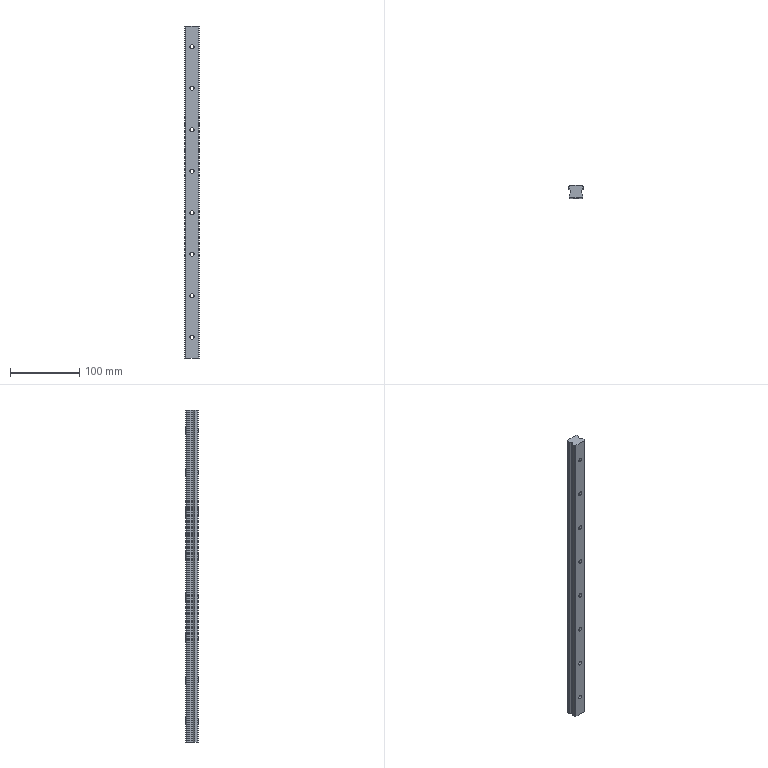Part | SolidWorks | features Chamfer 1, Extrusion 1, HoleWzd 1, LPattern 1 | 1 solid | 68 faces | box 20.703 x 18 x 480 mm | volume 151850 mm3 | cylinder 42 | plane 26 | commonest cylinder face diameters 6 x16 9.5 x16 2.4 x10